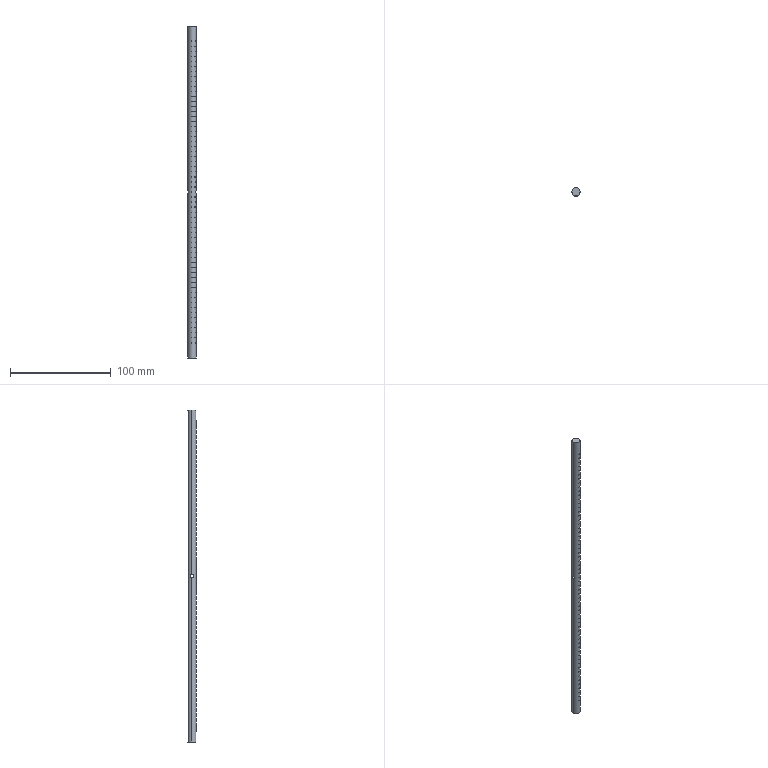Part | SolidWorks | features ICE 3, LPattern 2, Extrusion 1 | 1 solid | 310 faces | box 8 x 8 x 330 mm | volume 16519 mm3 | plane 245 | cylinder 65 | commonest cylinder face diameters 7.8 x61 3.2 x2 8 x2